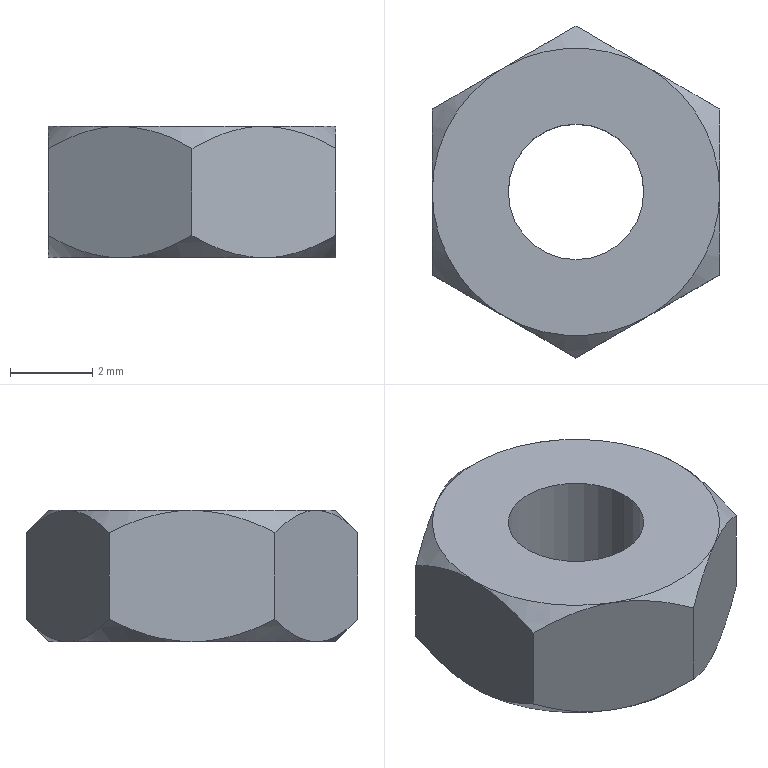Part | NX | 1 solid | 22 faces | box 7 x 8.083 x 3.2 mm | volume 107.132 mm3 | cone 12 | plane 8 | cylinder 2 | commonest cylinder face diameters 3.3 x2
STEP:
#1=CARTESIAN_POINT('',(1.75,-3.031,-1.6));
#2=VERTEX_POINT('',#1);
#3=CARTESIAN_POINT('',(3.5,0.,-1.6));
#4=VERTEX_POINT('',#3);
#5=CARTESIAN_POINT('',(0.,0.,-1.6));
#6=DIRECTION('',(0.,0.,1.));
#7=DIRECTION('',(0.5,-0.866,0.));
#8=AXIS2_PLACEMENT_3D('',#5,#6,#7);
#9=CIRCLE('',#8,3.5);
#10=EDGE_CURVE('',#2,#4,#9,.T.);
#11=ORIENTED_EDGE('',*,*,#10,.F.);
#12=CARTESIAN_POINT('',(-1.75,-3.031,-1.6));
#13=VERTEX_POINT('',#12);
#14=CARTESIAN_POINT('',(0.,0.,-1.6));
#15=DIRECTION('',(0.,0.,1.));
#16=DIRECTION('',(-0.5,-0.866,0.));
#17=AXIS2_PLACEMENT_3D('',#14,#15,#16);
#18=CIRCLE('',#17,3.5);
#19=EDGE_CURVE('',#13,#2,#18,.T.);
#20=ORIENTED_EDGE('',*,*,#19,.F.);
#21=CARTESIAN_POINT('',(-3.5,0.,-1.6));
#22=VERTEX_POINT('',#21);
#23=CARTESIAN_POINT('',(0.,0.,-1.6));
#24=DIRECTION('',(0.,0.,1.));
#25=DIRECTION('',(-1.,0.,0.));
#26=AXIS2_PLACEMENT_3D('',#23,#24,#25);
#27=CIRCLE('',#26,3.5);
#28=EDGE_CURVE('',#22,#13,#27,.T.);
#29=ORIENTED_EDGE('',*,*,#28,.F.);
#30=CARTESIAN_POINT('',(-1.75,3.031,-1.6));
#31=VERTEX_POINT('',#30);
#32=CARTESIAN_POINT('',(0.,0.,-1.6));
#33=DIRECTION('',(0.,0.,1.));
#34=DIRECTION('',(-0.5,0.866,0.));
#35=AXIS2_PLACEMENT_3D('',#32,#33,#34);
#36=CIRCLE('',#35,3.5);
#37=EDGE_CURVE('',#31,#22,#36,.T.);
#38=ORIENTED_EDGE('',*,*,#37,.F.);
#39=CARTESIAN_POINT('',(1.75,3.031,-1.6));
#40=VERTEX_POINT('',#39);
#41=CARTESIAN_POINT('',(0.,0.,-1.6));
#42=DIRECTION('',(0.,0.,1.));
#43=DIRECTION('',(0.5,0.866,0.));
#44=AXIS2_PLACEMENT_3D('',#41,#42,#43);
#45=CIRCLE('',#44,3.5);
#46=EDGE_CURVE('',#40,#31,#45,.T.);
#47=ORIENTED_EDGE('',*,*,#46,.F.);
#48=CARTESIAN_POINT('',(0.,0.,-1.6));
#49=DIRECTION('',(0.,0.,1.));
#50=DIRECTION('',(1.,0.,0.));
#51=AXIS2_PLACEMENT_3D('',#48,#49,#50);
#52=CIRCLE('',#51,3.5);
#53=EDGE_CURVE('',#4,#40,#52,.T.);
#54=ORIENTED_EDGE('',*,*,#53,.F.);
#55=EDGE_LOOP('',(#11,#20,#29,#38,#47,#54));
#56=FACE_BOUND('',#55,.T.);
#57=CARTESIAN_POINT('',(1.65,0.,-1.6));
#58=VERTEX_POINT('',#57);
#59=CARTESIAN_POINT('',(-1.65,0.,-1.6));
#60=VERTEX_POINT('',#59);
#61=CARTESIAN_POINT('',(0.,0.,-1.6));
#62=DIRECTION('',(0.,0.,-1.));
#63=DIRECTION('',(1.,0.,0.));
#64=AXIS2_PLACEMENT_3D('',#61,#62,#63);
#65=CIRCLE('',#64,1.65);
#66=EDGE_CURVE('',#58,#60,#65,.T.);
#67=ORIENTED_EDGE('',*,*,#66,.F.);
#68=CARTESIAN_POINT('',(0.,0.,-1.6));
#69=DIRECTION('',(0.,0.,-1.));
#70=DIRECTION('',(1.,0.,0.));
#71=AXIS2_PLACEMENT_3D('',#68,#69,#70);
#72=CIRCLE('',#71,1.65);
#73=EDGE_CURVE('',#60,#58,#72,.T.);
#74=ORIENTED_EDGE('',*,*,#73,.F.);
#75=EDGE_LOOP('',(#67,#74));
#76=FACE_BOUND('',#75,.T.);
#77=CARTESIAN_POINT('',(0.,0.,-1.6));
#78=DIRECTION('',(0.,0.,1.));
#79=DIRECTION('',(1.,0.,0.));
#80=AXIS2_PLACEMENT_3D('',#77,#78,#79);
#81=PLANE('',#80);
#82=ADVANCED_FACE('',(#56,#76),#81,.F.);
#83=CARTESIAN_POINT('',(3.5,-2.021,-1.059));
#84=VERTEX_POINT('',#83);
#85=CARTESIAN_POINT('',(1.75,-3.031,-1.6));
#86=CARTESIAN_POINT('',(2.303,-2.712,-1.6));
#87=CARTESIAN_POINT('',(2.867,-2.386,-1.424));
#88=CARTESIAN_POINT('',(3.5,-2.021,-1.059));
#89=B_SPLINE_CURVE_WITH_KNOTS('',3,(#85,#86,#87,#88),.UNSPECIFIED.,.F.,.F.,(4,4),(0.,1.),.UNSPECIFIED.);
#90=EDGE_CURVE('',#2,#84,#89,.T.);
#91=ORIENTED_EDGE('',*,*,#90,.F.);
#92=ORIENTED_EDGE('',*,*,#10,.T.);
#93=CARTESIAN_POINT('',(3.5,-2.021,-1.059));
#94=CARTESIAN_POINT('',(3.5,-1.292,-1.423));
#95=CARTESIAN_POINT('',(3.5,-0.6431,-1.6));
#96=CARTESIAN_POINT('',(3.5,0.,-1.6));
#97=B_SPLINE_CURVE_WITH_KNOTS('',3,(#93,#94,#95,#96),.UNSPECIFIED.,.F.,.F.,(4,4),(0.,1.),.UNSPECIFIED.);
#98=EDGE_CURVE('',#84,#4,#97,.T.);
#99=ORIENTED_EDGE('',*,*,#98,.F.);
#100=EDGE_LOOP('',(#91,#92,#99));
#101=FACE_BOUND('',#100,.T.);
#102=CARTESIAN_POINT('',(0.,0.,-1.329));
#103=DIRECTION('',(0.,0.,1.));
#104=DIRECTION('',(1.,0.,0.));
#105=AXIS2_PLACEMENT_3D('',#102,#103,#104);
#106=CONICAL_SURFACE('',#105,3.771,0.7854);
#107=ADVANCED_FACE('',(#101),#106,.T.);
#108=ORIENTED_EDGE('',*,*,#90,.T.);
#109=CARTESIAN_POINT('',(3.5,-2.021,1.059));
#110=VERTEX_POINT('',#109);
#111=CARTESIAN_POINT('',(3.5,-2.021,1.059));
#112=DIRECTION('',(0.,0.,-1.));
#113=VECTOR('',#112,1000.);
#114=LINE('',#111,#113);
#115=EDGE_CURVE('',#110,#84,#114,.T.);
#116=ORIENTED_EDGE('',*,*,#115,.F.);
#117=CARTESIAN_POINT('',(1.75,-3.031,1.6));
#118=VERTEX_POINT('',#117);
#119=CARTESIAN_POINT('',(3.5,-2.021,1.059));
#120=CARTESIAN_POINT('',(3.218,-2.183,1.221));
#121=CARTESIAN_POINT('',(2.75,-2.454,1.458));
#122=CARTESIAN_POINT('',(2.058,-2.853,1.6));
#123=CARTESIAN_POINT('',(1.75,-3.031,1.6));
#124=B_SPLINE_CURVE_WITH_KNOTS('',3,(#119,#120,#121,#122,#123),.UNSPECIFIED.,.F.,.F.,(4,1,4),(0.,0.5,1.),.UNSPECIFIED.);
#125=EDGE_CURVE('',#118,#110,#124,.F.);
#126=ORIENTED_EDGE('',*,*,#125,.F.);
#127=CARTESIAN_POINT('',(0.,-4.041,1.059));
#128=VERTEX_POINT('',#127);
#129=CARTESIAN_POINT('',(1.75,-3.031,1.6));
#130=CARTESIAN_POINT('',(1.197,-3.351,1.6));
#131=CARTESIAN_POINT('',(0.633,-3.676,1.424));
#132=CARTESIAN_POINT('',(0.,-4.041,1.059));
#133=B_SPLINE_CURVE_WITH_KNOTS('',3,(#129,#130,#131,#132),.UNSPECIFIED.,.F.,.F.,(4,4),(0.,1.),.UNSPECIFIED.);
#134=EDGE_CURVE('',#118,#128,#133,.T.);
#135=ORIENTED_EDGE('',*,*,#134,.T.);
#136=CARTESIAN_POINT('',(0.,-4.041,-1.059));
#137=VERTEX_POINT('',#136);
#138=CARTESIAN_POINT('',(0.,-4.041,1.059));
#139=DIRECTION('',(0.,0.,-1.));
#140=VECTOR('',#139,1000.);
#141=LINE('',#138,#140);
#142=EDGE_CURVE('',#128,#137,#141,.T.);
#143=ORIENTED_EDGE('',*,*,#142,.T.);
#144=CARTESIAN_POINT('',(0.,-4.041,-1.059));
#145=CARTESIAN_POINT('',(0.06595,-4.003,-1.097));
#146=CARTESIAN_POINT('',(0.1955,-3.929,-1.168));
#147=CARTESIAN_POINT('',(0.382,-3.821,-1.262));
#148=CARTESIAN_POINT('',(0.5626,-3.717,-1.343));
#149=CARTESIAN_POINT('',(0.7385,-3.615,-1.412));
#150=CARTESIAN_POINT('',(0.9112,-3.515,-1.47));
#151=CARTESIAN_POINT('',(1.081,-3.417,-1.518));
#152=CARTESIAN_POINT('',(1.25,-3.32,-1.554));
#153=CARTESIAN_POINT('',(1.417,-3.223,-1.581));
#154=CARTESIAN_POINT('',(1.584,-3.127,-1.596));
#155=CARTESIAN_POINT('',(1.695,-3.063,-1.6));
#156=CARTESIAN_POINT('',(1.75,-3.031,-1.6));
#157=B_SPLINE_CURVE_WITH_KNOTS('',3,(#144,#145,#146,#147,#148,#149,#150,#151,#152,#153,#154,#155,#156),.UNSPECIFIED.,.F.,.F.,(4,1,1,1,1,1,1,1,1,1,4),(0.,0.1,0.2,0.3,0.4,0.5,0.6,0.7,0.8,0.9,1.),.UNSPECIFIED.);
#158=EDGE_CURVE('',#137,#2,#157,.T.);
#159=ORIENTED_EDGE('',*,*,#158,.T.);
#160=EDGE_LOOP('',(#108,#116,#126,#135,#143,#159));
#161=FACE_BOUND('',#160,.T.);
#162=CARTESIAN_POINT('',(0.,-4.041,-1.6));
#163=DIRECTION('',(0.5,-0.866,0.));
#164=DIRECTION('',(0.,0.,-1.));
#165=AXIS2_PLACEMENT_3D('',#162,#163,#164);
#166=PLANE('',#165);
#167=ADVANCED_FACE('',(#161),#166,.T.);
#168=CARTESIAN_POINT('',(-1.75,-3.031,-1.6));
#169=CARTESIAN_POINT('',(-1.197,-3.35,-1.6));
#170=CARTESIAN_POINT('',(-0.633,-3.676,-1.424));
#171=CARTESIAN_POINT('',(0.,-4.041,-1.059));
#172=B_SPLINE_CURVE_WITH_KNOTS('',3,(#168,#169,#170,#171),.UNSPECIFIED.,.F.,.F.,(4,4),(0.,1.),.UNSPECIFIED.);
#173=EDGE_CURVE('',#13,#137,#172,.T.);
#174=ORIENTED_EDGE('',*,*,#173,.F.);
#175=ORIENTED_EDGE('',*,*,#19,.T.);
#176=ORIENTED_EDGE('',*,*,#158,.F.);
#177=EDGE_LOOP('',(#174,#175,#176));
#178=FACE_BOUND('',#177,.T.);
#179=CARTESIAN_POINT('',(0.,0.,-1.329));
#180=DIRECTION('',(0.,0.,1.));
#181=DIRECTION('',(1.,0.,0.));
#182=AXIS2_PLACEMENT_3D('',#179,#180,#181);
#183=CONICAL_SURFACE('',#182,3.771,0.7854);
#184=ADVANCED_FACE('',(#178),#183,.T.);
#185=ORIENTED_EDGE('',*,*,#173,.T.);
#186=ORIENTED_EDGE('',*,*,#142,.F.);
#187=CARTESIAN_POINT('',(-1.75,-3.031,1.6));
#188=VERTEX_POINT('',#187);
#189=CARTESIAN_POINT('',(0.,-4.041,1.059));
#190=CARTESIAN_POINT('',(-0.2817,-3.879,1.221));
#191=CARTESIAN_POINT('',(-0.7496,-3.609,1.458));
#192=CARTESIAN_POINT('',(-1.442,-3.209,1.6));
#193=CARTESIAN_POINT('',(-1.75,-3.031,1.6));
#194=B_SPLINE_CURVE_WITH_KNOTS('',3,(#189,#190,#191,#192,#193),.UNSPECIFIED.,.F.,.F.,(4,1,4),(0.,0.5,1.),.UNSPECIFIED.);
#195=EDGE_CURVE('',#188,#128,#194,.F.);
#196=ORIENTED_EDGE('',*,*,#195,.F.);
#197=CARTESIAN_POINT('',(-3.5,-2.021,1.059));
#198=VERTEX_POINT('',#197);
#199=CARTESIAN_POINT('',(-1.75,-3.031,1.6));
#200=CARTESIAN_POINT('',(-2.303,-2.712,1.6));
#201=CARTESIAN_POINT('',(-2.867,-2.386,1.424));
#202=CARTESIAN_POINT('',(-3.5,-2.021,1.059));
#203=B_SPLINE_CURVE_WITH_KNOTS('',3,(#199,#200,#201,#202),.UNSPECIFIED.,.F.,.F.,(4,4),(0.,1.),.UNSPECIFIED.);
#204=EDGE_CURVE('',#188,#198,#203,.T.);
#205=ORIENTED_EDGE('',*,*,#204,.T.);
#206=CARTESIAN_POINT('',(-3.5,-2.021,-1.059));
#207=VERTEX_POINT('',#206);
#208=CARTESIAN_POINT('',(-3.5,-2.021,1.059));
#209=DIRECTION('',(0.,0.,-1.));
#210=VECTOR('',#209,1000.);
#211=LINE('',#208,#210);
#212=EDGE_CURVE('',#198,#207,#211,.T.);
#213=ORIENTED_EDGE('',*,*,#212,.T.);
#214=CARTESIAN_POINT('',(-3.5,-2.021,-1.059));
#215=CARTESIAN_POINT('',(-3.434,-2.059,-1.097));
#216=CARTESIAN_POINT('',(-3.304,-2.134,-1.168));
#217=CARTESIAN_POINT('',(-3.118,-2.241,-1.262));
#218=CARTESIAN_POINT('',(-2.937,-2.346,-1.343));
#219=CARTESIAN_POINT('',(-2.761,-2.447,-1.412));
#220=CARTESIAN_POINT('',(-2.589,-2.547,-1.47));
#221=CARTESIAN_POINT('',(-2.419,-2.645,-1.518));
#222=CARTESIAN_POINT('',(-2.25,-2.742,-1.554));
#223=CARTESIAN_POINT('',(-2.083,-2.839,-1.581));
#224=CARTESIAN_POINT('',(-1.916,-2.935,-1.596));
#225=CARTESIAN_POINT('',(-1.805,-2.999,-1.6));
#226=CARTESIAN_POINT('',(-1.75,-3.031,-1.6));
#227=B_SPLINE_CURVE_WITH_KNOTS('',3,(#214,#215,#216,#217,#218,#219,#220,#221,#222,#223,#224,#225,#226),.UNSPECIFIED.,.F.,.F.,(4,1,1,1,1,1,1,1,1,1,4),(0.,0.1,0.2,0.3,0.4,0.5,0.6,0.7,0.8,0.9,1.),.UNSPECIFIED.);
#228=EDGE_CURVE('',#207,#13,#227,.T.);
#229=ORIENTED_EDGE('',*,*,#228,.T.);
#230=EDGE_LOOP('',(#185,#186,#196,#205,#213,#229));
#231=FACE_BOUND('',#230,.T.);
#232=CARTESIAN_POINT('',(-3.5,-2.021,-1.6));
#233=DIRECTION('',(-0.5,-0.866,0.));
#234=DIRECTION('',(-0.866,0.5,0.));
#235=AXIS2_PLACEMENT_3D('',#232,#233,#234);
#236=PLANE('',#235);
#237=ADVANCED_FACE('',(#231),#236,.T.);
#238=CARTESIAN_POINT('',(-3.5,0.,-1.6));
#239=CARTESIAN_POINT('',(-3.5,-0.6387,-1.6));
#240=CARTESIAN_POINT('',(-3.5,-1.29,-1.424));
#241=CARTESIAN_POINT('',(-3.5,-2.021,-1.059));
#242=B_SPLINE_CURVE_WITH_KNOTS('',3,(#238,#239,#240,#241),.UNSPECIFIED.,.F.,.F.,(4,4),(0.,1.),.UNSPECIFIED.);
#243=EDGE_CURVE('',#22,#207,#242,.T.);
#244=ORIENTED_EDGE('',*,*,#243,.F.);
#245=ORIENTED_EDGE('',*,*,#28,.T.);
#246=ORIENTED_EDGE('',*,*,#228,.F.);
#247=EDGE_LOOP('',(#244,#245,#246));
#248=FACE_BOUND('',#247,.T.);
#249=CARTESIAN_POINT('',(0.,0.,-1.329));
#250=DIRECTION('',(0.,0.,1.));
#251=DIRECTION('',(1.,0.,0.));
#252=AXIS2_PLACEMENT_3D('',#249,#250,#251);
#253=CONICAL_SURFACE('',#252,3.771,0.7854);
#254=ADVANCED_FACE('',(#248),#253,.T.);
#255=ORIENTED_EDGE('',*,*,#243,.T.);
#256=ORIENTED_EDGE('',*,*,#212,.F.);
#257=CARTESIAN_POINT('',(-3.5,0.,1.6));
#258=VERTEX_POINT('',#257);
#259=CARTESIAN_POINT('',(-3.5,-2.021,1.059));
#260=CARTESIAN_POINT('',(-3.5,-1.692,1.223));
#261=CARTESIAN_POINT('',(-3.5,-1.139,1.463));
#262=CARTESIAN_POINT('',(-3.5,-0.3527,1.6));
#263=CARTESIAN_POINT('',(-3.5,0.,1.6));
#264=B_SPLINE_CURVE_WITH_KNOTS('',3,(#259,#260,#261,#262,#263),.UNSPECIFIED.,.F.,.F.,(4,1,4),(0.,0.5,1.),.UNSPECIFIED.);
#265=EDGE_CURVE('',#258,#198,#264,.F.);
#266=ORIENTED_EDGE('',*,*,#265,.F.);
#267=CARTESIAN_POINT('',(-3.5,2.021,1.059));
#268=VERTEX_POINT('',#267);
#269=CARTESIAN_POINT('',(-3.5,0.,1.6));
#270=CARTESIAN_POINT('',(-3.5,0.6387,1.6));
#271=CARTESIAN_POINT('',(-3.5,1.29,1.424));
#272=CARTESIAN_POINT('',(-3.5,2.021,1.059));
#273=B_SPLINE_CURVE_WITH_KNOTS('',3,(#269,#270,#271,#272),.UNSPECIFIED.,.F.,.F.,(4,4),(0.,1.),.UNSPECIFIED.);
#274=EDGE_CURVE('',#258,#268,#273,.T.);
#275=ORIENTED_EDGE('',*,*,#274,.T.);
#276=CARTESIAN_POINT('',(-3.5,2.021,-1.059));
#277=VERTEX_POINT('',#276);
#278=CARTESIAN_POINT('',(-3.5,2.021,1.059));
#279=DIRECTION('',(0.,0.,-1.));
#280=VECTOR('',#279,1000.);
#281=LINE('',#278,#280);
#282=EDGE_CURVE('',#268,#277,#281,.T.);
#283=ORIENTED_EDGE('',*,*,#282,.T.);
#284=CARTESIAN_POINT('',(-3.5,2.021,-1.059));
#285=CARTESIAN_POINT('',(-3.5,1.292,-1.423));
#286=CARTESIAN_POINT('',(-3.5,0.6431,-1.6));
#287=CARTESIAN_POINT('',(-3.5,0.,-1.6));
#288=B_SPLINE_CURVE_WITH_KNOTS('',3,(#284,#285,#286,#287),.UNSPECIFIED.,.F.,.F.,(4,4),(0.,1.),.UNSPECIFIED.);
#289=EDGE_CURVE('',#277,#22,#288,.T.);
#290=ORIENTED_EDGE('',*,*,#289,.T.);
#291=EDGE_LOOP('',(#255,#256,#266,#275,#283,#290));
#292=FACE_BOUND('',#291,.T.);
#293=CARTESIAN_POINT('',(-3.5,2.021,-1.6));
#294=DIRECTION('',(-1.,0.,0.));
#295=DIRECTION('',(0.,0.,1.));
#296=AXIS2_PLACEMENT_3D('',#293,#294,#295);
#297=PLANE('',#296);
#298=ADVANCED_FACE('',(#292),#297,.T.);
#299=CARTESIAN_POINT('',(-1.75,3.031,-1.6));
#300=CARTESIAN_POINT('',(-2.303,2.712,-1.6));
#301=CARTESIAN_POINT('',(-2.867,2.386,-1.424));
#302=CARTESIAN_POINT('',(-3.5,2.021,-1.059));
#303=B_SPLINE_CURVE_WITH_KNOTS('',3,(#299,#300,#301,#302),.UNSPECIFIED.,.F.,.F.,(4,4),(0.,1.),.UNSPECIFIED.);
#304=EDGE_CURVE('',#31,#277,#303,.T.);
#305=ORIENTED_EDGE('',*,*,#304,.F.);
#306=ORIENTED_EDGE('',*,*,#37,.T.);
#307=ORIENTED_EDGE('',*,*,#289,.F.);
#308=EDGE_LOOP('',(#305,#306,#307));
#309=FACE_BOUND('',#308,.T.);
#310=CARTESIAN_POINT('',(0.,0.,-1.329));
#311=DIRECTION('',(0.,0.,1.));
#312=DIRECTION('',(1.,0.,0.));
#313=AXIS2_PLACEMENT_3D('',#310,#311,#312);
#314=CONICAL_SURFACE('',#313,3.771,0.7854);
#315=ADVANCED_FACE('',(#309),#314,.T.);
#316=ORIENTED_EDGE('',*,*,#304,.T.);
#317=ORIENTED_EDGE('',*,*,#282,.F.);
#318=CARTESIAN_POINT('',(-1.75,3.031,1.6));
#319=VERTEX_POINT('',#318);
#320=CARTESIAN_POINT('',(-3.5,2.021,1.059));
#321=CARTESIAN_POINT('',(-3.218,2.183,1.221));
#322=CARTESIAN_POINT('',(-2.75,2.454,1.458));
#323=CARTESIAN_POINT('',(-2.058,2.853,1.6));
#324=CARTESIAN_POINT('',(-1.75,3.031,1.6));
#325=B_SPLINE_CURVE_WITH_KNOTS('',3,(#320,#321,#322,#323,#324),.UNSPECIFIED.,.F.,.F.,(4,1,4),(0.,0.5,1.),.UNSPECIFIED.);
#326=EDGE_CURVE('',#319,#268,#325,.F.);
#327=ORIENTED_EDGE('',*,*,#326,.F.);
#328=CARTESIAN_POINT('',(0.,4.041,1.059));
#329=VERTEX_POINT('',#328);
#330=CARTESIAN_POINT('',(-1.75,3.031,1.6));
#331=CARTESIAN_POINT('',(-1.197,3.351,1.6));
#332=CARTESIAN_POINT('',(-0.633,3.676,1.424));
#333=CARTESIAN_POINT('',(0.,4.041,1.059));
#334=B_SPLINE_CURVE_WITH_KNOTS('',3,(#330,#331,#332,#333),.UNSPECIFIED.,.F.,.F.,(4,4),(0.,1.),.UNSPECIFIED.);
#335=EDGE_CURVE('',#319,#329,#334,.T.);
#336=ORIENTED_EDGE('',*,*,#335,.T.);
#337=CARTESIAN_POINT('',(0.,4.041,-1.059));
#338=VERTEX_POINT('',#337);
#339=CARTESIAN_POINT('',(0.,4.041,1.059));
#340=DIRECTION('',(0.,0.,-1.));
#341=VECTOR('',#340,1000.);
#342=LINE('',#339,#341);
#343=EDGE_CURVE('',#329,#338,#342,.T.);
#344=ORIENTED_EDGE('',*,*,#343,.T.);
#345=CARTESIAN_POINT('',(0.,4.041,-1.059));
#346=CARTESIAN_POINT('',(-0.06595,4.003,-1.097));
#347=CARTESIAN_POINT('',(-0.1955,3.929,-1.168));
#348=CARTESIAN_POINT('',(-0.382,3.821,-1.262));
#349=CARTESIAN_POINT('',(-0.5626,3.717,-1.343));
#350=CARTESIAN_POINT('',(-0.7385,3.615,-1.412));
#351=CARTESIAN_POINT('',(-0.9112,3.515,-1.47));
#352=CARTESIAN_POINT('',(-1.081,3.417,-1.518));
#353=CARTESIAN_POINT('',(-1.25,3.32,-1.554));
#354=CARTESIAN_POINT('',(-1.417,3.223,-1.581));
#355=CARTESIAN_POINT('',(-1.584,3.127,-1.596));
#356=CARTESIAN_POINT('',(-1.695,3.063,-1.6));
#357=CARTESIAN_POINT('',(-1.75,3.031,-1.6));
#358=B_SPLINE_CURVE_WITH_KNOTS('',3,(#345,#346,#347,#348,#349,#350,#351,#352,#353,#354,#355,#356,#357),.UNSPECIFIED.,.F.,.F.,(4,1,1,1,1,1,1,1,1,1,4),(0.,0.1,0.2,0.3,0.4,0.5,0.6,0.7,0.8,0.9,1.),.UNSPECIFIED.);
#359=EDGE_CURVE('',#338,#31,#358,.T.);
#360=ORIENTED_EDGE('',*,*,#359,.T.);
#361=EDGE_LOOP('',(#316,#317,#327,#336,#344,#360));
#362=FACE_BOUND('',#361,.T.);
#363=CARTESIAN_POINT('',(0.,4.041,-1.6));
#364=DIRECTION('',(-0.5,0.866,0.));
#365=DIRECTION('',(0.,0.,1.));
#366=AXIS2_PLACEMENT_3D('',#363,#364,#365);
#367=PLANE('',#366);
#368=ADVANCED_FACE('',(#362),#367,.T.);
#369=CARTESIAN_POINT('',(1.75,3.031,-1.6));
#370=CARTESIAN_POINT('',(1.197,3.35,-1.6));
#371=CARTESIAN_POINT('',(0.633,3.676,-1.424));
#372=CARTESIAN_POINT('',(0.,4.041,-1.059));
#373=B_SPLINE_CURVE_WITH_KNOTS('',3,(#369,#370,#371,#372),.UNSPECIFIED.,.F.,.F.,(4,4),(0.,1.),.UNSPECIFIED.);
#374=EDGE_CURVE('',#40,#338,#373,.T.);
#375=ORIENTED_EDGE('',*,*,#374,.F.);
#376=ORIENTED_EDGE('',*,*,#46,.T.);
#377=ORIENTED_EDGE('',*,*,#359,.F.);
#378=EDGE_LOOP('',(#375,#376,#377));
#379=FACE_BOUND('',#378,.T.);
#380=CARTESIAN_POINT('',(0.,0.,-1.329));
#381=DIRECTION('',(0.,0.,1.));
#382=DIRECTION('',(1.,0.,0.));
#383=AXIS2_PLACEMENT_3D('',#380,#381,#382);
#384=CONICAL_SURFACE('',#383,3.771,0.7854);
#385=ADVANCED_FACE('',(#379),#384,.T.);
#386=ORIENTED_EDGE('',*,*,#374,.T.);
#387=ORIENTED_EDGE('',*,*,#343,.F.);
#388=CARTESIAN_POINT('',(1.75,3.031,1.6));
#389=VERTEX_POINT('',#388);
#390=CARTESIAN_POINT('',(0.,4.041,1.059));
#391=CARTESIAN_POINT('',(0.2817,3.879,1.221));
#392=CARTESIAN_POINT('',(0.7496,3.609,1.458));
#393=CARTESIAN_POINT('',(1.442,3.209,1.6));
#394=CARTESIAN_POINT('',(1.75,3.031,1.6));
#395=B_SPLINE_CURVE_WITH_KNOTS('',3,(#390,#391,#392,#393,#394),.UNSPECIFIED.,.F.,.F.,(4,1,4),(0.,0.5,1.),.UNSPECIFIED.);
#396=EDGE_CURVE('',#389,#329,#395,.F.);
#397=ORIENTED_EDGE('',*,*,#396,.F.);
#398=CARTESIAN_POINT('',(3.5,2.021,1.059));
#399=VERTEX_POINT('',#398);
#400=CARTESIAN_POINT('',(1.75,3.031,1.6));
#401=CARTESIAN_POINT('',(2.303,2.712,1.6));
#402=CARTESIAN_POINT('',(2.867,2.386,1.424));
#403=CARTESIAN_POINT('',(3.5,2.021,1.059));
#404=B_SPLINE_CURVE_WITH_KNOTS('',3,(#400,#401,#402,#403),.UNSPECIFIED.,.F.,.F.,(4,4),(0.,1.),.UNSPECIFIED.);
#405=EDGE_CURVE('',#389,#399,#404,.T.);
#406=ORIENTED_EDGE('',*,*,#405,.T.);
#407=CARTESIAN_POINT('',(3.5,2.021,-1.059));
#408=VERTEX_POINT('',#407);
#409=CARTESIAN_POINT('',(3.5,2.021,1.059));
#410=DIRECTION('',(0.,0.,-1.));
#411=VECTOR('',#410,1000.);
#412=LINE('',#409,#411);
#413=EDGE_CURVE('',#399,#408,#412,.T.);
#414=ORIENTED_EDGE('',*,*,#413,.T.);
#415=CARTESIAN_POINT('',(3.5,2.021,-1.059));
#416=CARTESIAN_POINT('',(3.434,2.059,-1.097));
#417=CARTESIAN_POINT('',(3.304,2.134,-1.168));
#418=CARTESIAN_POINT('',(3.118,2.241,-1.262));
#419=CARTESIAN_POINT('',(2.937,2.346,-1.343));
#420=CARTESIAN_POINT('',(2.761,2.447,-1.412));
#421=CARTESIAN_POINT('',(2.589,2.547,-1.47));
#422=CARTESIAN_POINT('',(2.419,2.645,-1.518));
#423=CARTESIAN_POINT('',(2.25,2.742,-1.554));
#424=CARTESIAN_POINT('',(2.083,2.839,-1.581));
#425=CARTESIAN_POINT('',(1.916,2.935,-1.596));
#426=CARTESIAN_POINT('',(1.805,2.999,-1.6));
#427=CARTESIAN_POINT('',(1.75,3.031,-1.6));
#428=B_SPLINE_CURVE_WITH_KNOTS('',3,(#415,#416,#417,#418,#419,#420,#421,#422,#423,#424,#425,#426,#427),.UNSPECIFIED.,.F.,.F.,(4,1,1,1,1,1,1,1,1,1,4),(0.,0.1,0.2,0.3,0.4,0.5,0.6,0.7,0.8,0.9,1.),.UNSPECIFIED.);
#429=EDGE_CURVE('',#408,#40,#428,.T.);
#430=ORIENTED_EDGE('',*,*,#429,.T.);
#431=EDGE_LOOP('',(#386,#387,#397,#406,#414,#430));
#432=FACE_BOUND('',#431,.T.);
#433=CARTESIAN_POINT('',(3.5,2.021,-1.6));
#434=DIRECTION('',(0.5,0.866,0.));
#435=DIRECTION('',(0.,0.,-1.));
#436=AXIS2_PLACEMENT_3D('',#433,#434,#435);
#437=PLANE('',#436);
#438=ADVANCED_FACE('',(#432),#437,.T.);
#439=CARTESIAN_POINT('',(3.5,0.,-1.6));
#440=CARTESIAN_POINT('',(3.5,0.6387,-1.6));
#441=CARTESIAN_POINT('',(3.5,1.29,-1.424));
#442=CARTESIAN_POINT('',(3.5,2.021,-1.059));
#443=B_SPLINE_CURVE_WITH_KNOTS('',3,(#439,#440,#441,#442),.UNSPECIFIED.,.F.,.F.,(4,4),(0.,1.),.UNSPECIFIED.);
#444=EDGE_CURVE('',#4,#408,#443,.T.);
#445=ORIENTED_EDGE('',*,*,#444,.F.);
#446=ORIENTED_EDGE('',*,*,#53,.T.);
#447=ORIENTED_EDGE('',*,*,#429,.F.);
#448=EDGE_LOOP('',(#445,#446,#447));
#449=FACE_BOUND('',#448,.T.);
#450=CARTESIAN_POINT('',(0.,0.,-1.329));
#451=DIRECTION('',(0.,0.,1.));
#452=DIRECTION('',(1.,0.,0.));
#453=AXIS2_PLACEMENT_3D('',#450,#451,#452);
#454=CONICAL_SURFACE('',#453,3.771,0.7854);
#455=ADVANCED_FACE('',(#449),#454,.T.);
#456=ORIENTED_EDGE('',*,*,#98,.T.);
#457=ORIENTED_EDGE('',*,*,#444,.T.);
#458=ORIENTED_EDGE('',*,*,#413,.F.);
#459=CARTESIAN_POINT('',(3.5,0.,1.6));
#460=VERTEX_POINT('',#459);
#461=CARTESIAN_POINT('',(3.5,2.021,1.059));
#462=CARTESIAN_POINT('',(3.5,1.692,1.223));
#463=CARTESIAN_POINT('',(3.5,1.139,1.463));
#464=CARTESIAN_POINT('',(3.5,0.3527,1.6));
#465=CARTESIAN_POINT('',(3.5,0.,1.6));
#466=B_SPLINE_CURVE_WITH_KNOTS('',3,(#461,#462,#463,#464,#465),.UNSPECIFIED.,.F.,.F.,(4,1,4),(0.,0.5,1.),.UNSPECIFIED.);
#467=EDGE_CURVE('',#460,#399,#466,.F.);
#468=ORIENTED_EDGE('',*,*,#467,.F.);
#469=CARTESIAN_POINT('',(3.5,0.,1.6));
#470=CARTESIAN_POINT('',(3.5,-0.6387,1.6));
#471=CARTESIAN_POINT('',(3.5,-1.29,1.424));
#472=CARTESIAN_POINT('',(3.5,-2.021,1.059));
#473=B_SPLINE_CURVE_WITH_KNOTS('',3,(#469,#470,#471,#472),.UNSPECIFIED.,.F.,.F.,(4,4),(0.,1.),.UNSPECIFIED.);
#474=EDGE_CURVE('',#460,#110,#473,.T.);
#475=ORIENTED_EDGE('',*,*,#474,.T.);
#476=ORIENTED_EDGE('',*,*,#115,.T.);
#477=EDGE_LOOP('',(#456,#457,#458,#468,#475,#476));
#478=FACE_BOUND('',#477,.T.);
#479=CARTESIAN_POINT('',(3.5,-2.021,-1.6));
#480=DIRECTION('',(1.,0.,0.));
#481=DIRECTION('',(0.,1.,0.));
#482=AXIS2_PLACEMENT_3D('',#479,#480,#481);
#483=PLANE('',#482);
#484=ADVANCED_FACE('',(#478),#483,.T.);
#485=ORIENTED_EDGE('',*,*,#474,.F.);
#486=CARTESIAN_POINT('',(0.,0.,1.6));
#487=DIRECTION('',(0.,0.,-1.));
#488=DIRECTION('',(1.,0.,0.));
#489=AXIS2_PLACEMENT_3D('',#486,#487,#488);
#490=CIRCLE('',#489,3.5);
#491=EDGE_CURVE('',#460,#118,#490,.T.);
#492=ORIENTED_EDGE('',*,*,#491,.T.);
#493=ORIENTED_EDGE('',*,*,#125,.T.);
#494=EDGE_LOOP('',(#485,#492,#493));
#495=FACE_BOUND('',#494,.T.);
#496=CARTESIAN_POINT('',(0.,0.,1.329));
#497=DIRECTION('',(0.,0.,-1.));
#498=DIRECTION('',(-1.,0.,0.));
#499=AXIS2_PLACEMENT_3D('',#496,#497,#498);
#500=CONICAL_SURFACE('',#499,3.771,0.7854);
#501=ADVANCED_FACE('',(#495),#500,.T.);
#502=ORIENTED_EDGE('',*,*,#491,.F.);
#503=CARTESIAN_POINT('',(0.,0.,1.6));
#504=DIRECTION('',(0.,0.,-1.));
#505=DIRECTION('',(0.5,0.866,0.));
#506=AXIS2_PLACEMENT_3D('',#503,#504,#505);
#507=CIRCLE('',#506,3.5);
#508=EDGE_CURVE('',#389,#460,#507,.T.);
#509=ORIENTED_EDGE('',*,*,#508,.F.);
#510=CARTESIAN_POINT('',(0.,0.,1.6));
#511=DIRECTION('',(0.,0.,-1.));
#512=DIRECTION('',(-0.5,0.866,0.));
#513=AXIS2_PLACEMENT_3D('',#510,#511,#512);
#514=CIRCLE('',#513,3.5);
#515=EDGE_CURVE('',#319,#389,#514,.T.);
#516=ORIENTED_EDGE('',*,*,#515,.F.);
#517=CARTESIAN_POINT('',(0.,0.,1.6));
#518=DIRECTION('',(0.,0.,-1.));
#519=DIRECTION('',(-1.,0.,0.));
#520=AXIS2_PLACEMENT_3D('',#517,#518,#519);
#521=CIRCLE('',#520,3.5);
#522=EDGE_CURVE('',#258,#319,#521,.T.);
#523=ORIENTED_EDGE('',*,*,#522,.F.);
#524=CARTESIAN_POINT('',(0.,0.,1.6));
#525=DIRECTION('',(0.,0.,-1.));
#526=DIRECTION('',(-0.5,-0.866,0.));
#527=AXIS2_PLACEMENT_3D('',#524,#525,#526);
#528=CIRCLE('',#527,3.5);
#529=EDGE_CURVE('',#188,#258,#528,.T.);
#530=ORIENTED_EDGE('',*,*,#529,.F.);
#531=CARTESIAN_POINT('',(0.,0.,1.6));
#532=DIRECTION('',(0.,0.,-1.));
#533=DIRECTION('',(0.5,-0.866,0.));
#534=AXIS2_PLACEMENT_3D('',#531,#532,#533);
#535=CIRCLE('',#534,3.5);
#536=EDGE_CURVE('',#118,#188,#535,.T.);
#537=ORIENTED_EDGE('',*,*,#536,.F.);
#538=EDGE_LOOP('',(#502,#509,#516,#523,#530,#537));
#539=FACE_BOUND('',#538,.T.);
#540=CARTESIAN_POINT('',(1.65,0.,1.6));
#541=VERTEX_POINT('',#540);
#542=CARTESIAN_POINT('',(-1.65,0.,1.6));
#543=VERTEX_POINT('',#542);
#544=CARTESIAN_POINT('',(0.,0.,1.6));
#545=DIRECTION('',(0.,0.,1.));
#546=DIRECTION('',(-1.,0.,0.));
#547=AXIS2_PLACEMENT_3D('',#544,#545,#546);
#548=CIRCLE('',#547,1.65);
#549=EDGE_CURVE('',#541,#543,#548,.T.);
#550=ORIENTED_EDGE('',*,*,#549,.F.);
#551=CARTESIAN_POINT('',(0.,0.,1.6));
#552=DIRECTION('',(0.,0.,1.));
#553=DIRECTION('',(-1.,0.,0.));
#554=AXIS2_PLACEMENT_3D('',#551,#552,#553);
#555=CIRCLE('',#554,1.65);
#556=EDGE_CURVE('',#543,#541,#555,.T.);
#557=ORIENTED_EDGE('',*,*,#556,.F.);
#558=EDGE_LOOP('',(#550,#557));
#559=FACE_BOUND('',#558,.T.);
#560=CARTESIAN_POINT('',(0.,0.,1.6));
#561=DIRECTION('',(0.,0.,1.));
#562=DIRECTION('',(1.,0.,0.));
#563=AXIS2_PLACEMENT_3D('',#560,#561,#562);
#564=PLANE('',#563);
#565=ADVANCED_FACE('',(#539,#559),#564,.T.);
#566=ORIENTED_EDGE('',*,*,#134,.F.);
#567=ORIENTED_EDGE('',*,*,#536,.T.);
#568=ORIENTED_EDGE('',*,*,#195,.T.);
#569=EDGE_LOOP('',(#566,#567,#568));
#570=FACE_BOUND('',#569,.T.);
#571=CARTESIAN_POINT('',(0.,0.,1.329));
#572=DIRECTION('',(0.,0.,-1.));
#573=DIRECTION('',(-1.,0.,0.));
#574=AXIS2_PLACEMENT_3D('',#571,#572,#573);
#575=CONICAL_SURFACE('',#574,3.771,0.7854);
#576=ADVANCED_FACE('',(#570),#575,.T.);
#577=ORIENTED_EDGE('',*,*,#204,.F.);
#578=ORIENTED_EDGE('',*,*,#529,.T.);
#579=ORIENTED_EDGE('',*,*,#265,.T.);
#580=EDGE_LOOP('',(#577,#578,#579));
#581=FACE_BOUND('',#580,.T.);
#582=CARTESIAN_POINT('',(0.,0.,1.329));
#583=DIRECTION('',(0.,0.,-1.));
#584=DIRECTION('',(-1.,0.,0.));
#585=AXIS2_PLACEMENT_3D('',#582,#583,#584);
#586=CONICAL_SURFACE('',#585,3.771,0.7854);
#587=ADVANCED_FACE('',(#581),#586,.T.);
#588=ORIENTED_EDGE('',*,*,#274,.F.);
#589=ORIENTED_EDGE('',*,*,#522,.T.);
#590=ORIENTED_EDGE('',*,*,#326,.T.);
#591=EDGE_LOOP('',(#588,#589,#590));
#592=FACE_BOUND('',#591,.T.);
#593=CARTESIAN_POINT('',(0.,0.,1.329));
#594=DIRECTION('',(0.,0.,-1.));
#595=DIRECTION('',(-1.,0.,0.));
#596=AXIS2_PLACEMENT_3D('',#593,#594,#595);
#597=CONICAL_SURFACE('',#596,3.771,0.7854);
#598=ADVANCED_FACE('',(#592),#597,.T.);
#599=ORIENTED_EDGE('',*,*,#335,.F.);
#600=ORIENTED_EDGE('',*,*,#515,.T.);
#601=ORIENTED_EDGE('',*,*,#396,.T.);
#602=EDGE_LOOP('',(#599,#600,#601));
#603=FACE_BOUND('',#602,.T.);
#604=CARTESIAN_POINT('',(0.,0.,1.329));
#605=DIRECTION('',(0.,0.,-1.));
#606=DIRECTION('',(-1.,0.,0.));
#607=AXIS2_PLACEMENT_3D('',#604,#605,#606);
#608=CONICAL_SURFACE('',#607,3.771,0.7854);
#609=ADVANCED_FACE('',(#603),#608,.T.);
#610=ORIENTED_EDGE('',*,*,#405,.F.);
#611=ORIENTED_EDGE('',*,*,#508,.T.);
#612=ORIENTED_EDGE('',*,*,#467,.T.);
#613=EDGE_LOOP('',(#610,#611,#612));
#614=FACE_BOUND('',#613,.T.);
#615=CARTESIAN_POINT('',(0.,0.,1.329));
#616=DIRECTION('',(0.,0.,-1.));
#617=DIRECTION('',(-1.,0.,0.));
#618=AXIS2_PLACEMENT_3D('',#615,#616,#617);
#619=CONICAL_SURFACE('',#618,3.771,0.7854);
#620=ADVANCED_FACE('',(#614),#619,.T.);
#621=ORIENTED_EDGE('',*,*,#66,.T.);
#622=CARTESIAN_POINT('',(-1.65,0.,1.6));
#623=DIRECTION('',(0.,0.,-1.));
#624=VECTOR('',#623,1000.);
#625=LINE('',#622,#624);
#626=EDGE_CURVE('',#60,#543,#625,.F.);
#627=ORIENTED_EDGE('',*,*,#626,.T.);
#628=ORIENTED_EDGE('',*,*,#556,.T.);
#629=CARTESIAN_POINT('',(1.65,0.,1.6));
#630=DIRECTION('',(0.,0.,-1.));
#631=VECTOR('',#630,1000.);
#632=LINE('',#629,#631);
#633=EDGE_CURVE('',#58,#541,#632,.F.);
#634=ORIENTED_EDGE('',*,*,#633,.F.);
#635=EDGE_LOOP('',(#621,#627,#628,#634));
#636=FACE_BOUND('',#635,.T.);
#637=CARTESIAN_POINT('',(0.,0.,1.6));
#638=DIRECTION('',(0.,0.,-1.));
#639=DIRECTION('',(-1.,0.,0.));
#640=AXIS2_PLACEMENT_3D('',#637,#638,#639);
#641=CYLINDRICAL_SURFACE('',#640,1.65);
#642=ADVANCED_FACE('',(#636),#641,.F.);
#643=ORIENTED_EDGE('',*,*,#549,.T.);
#644=ORIENTED_EDGE('',*,*,#626,.F.);
#645=ORIENTED_EDGE('',*,*,#73,.T.);
#646=ORIENTED_EDGE('',*,*,#633,.T.);
#647=EDGE_LOOP('',(#643,#644,#645,#646));
#648=FACE_BOUND('',#647,.T.);
#649=CARTESIAN_POINT('',(0.,0.,1.6));
#650=DIRECTION('',(0.,0.,-1.));
#651=DIRECTION('',(-1.,0.,0.));
#652=AXIS2_PLACEMENT_3D('',#649,#650,#651);
#653=CYLINDRICAL_SURFACE('',#652,1.65);
#654=ADVANCED_FACE('',(#648),#653,.F.);
#655=CLOSED_SHELL('',(#82,#107,#167,#184,#237,#254,#298,#315,#368,#385,#438,#455,#484,#501,#565,#576,#587,#598,#609,#620,#642,#654));
#656=MANIFOLD_SOLID_BREP('',#655);
#657=(LENGTH_UNIT()NAMED_UNIT(*)SI_UNIT(.MILLI.,.METRE.));
#658=UNCERTAINTY_MEASURE_WITH_UNIT(LENGTH_MEASURE(0.0508),#657,'','');
#659=(NAMED_UNIT(*)PLANE_ANGLE_UNIT()SI_UNIT($,.RADIAN.));
#660=(NAMED_UNIT(*)SI_UNIT($,.STERADIAN.)SOLID_ANGLE_UNIT());
#661=(GEOMETRIC_REPRESENTATION_CONTEXT(3)GLOBAL_UNCERTAINTY_ASSIGNED_CONTEXT((#658))GLOBAL_UNIT_ASSIGNED_CONTEXT((#657,#659,#660))REPRESENTATION_CONTEXT('',''));
#662=ADVANCED_BREP_SHAPE_REPRESENTATION('',(#656),#661);